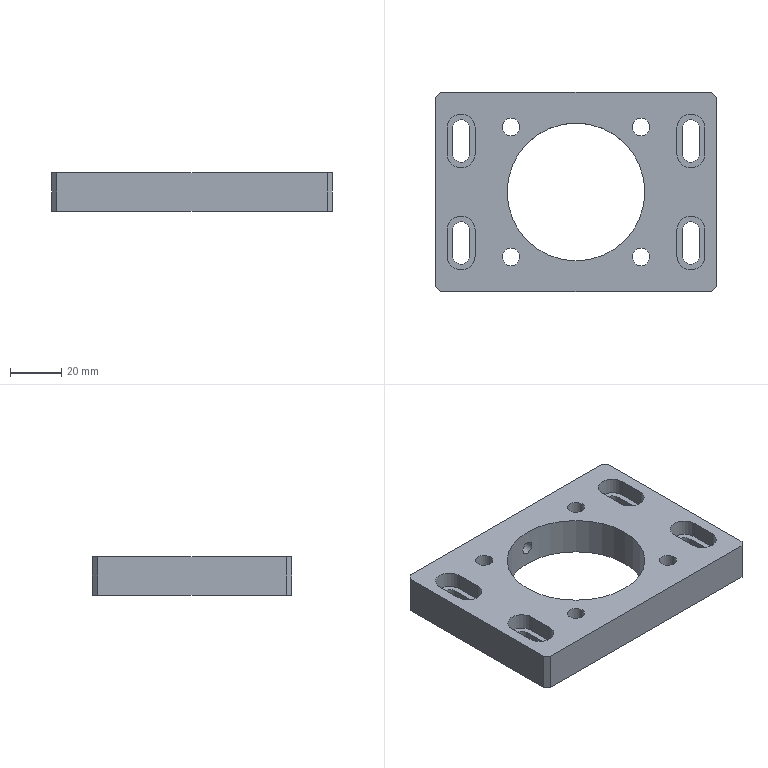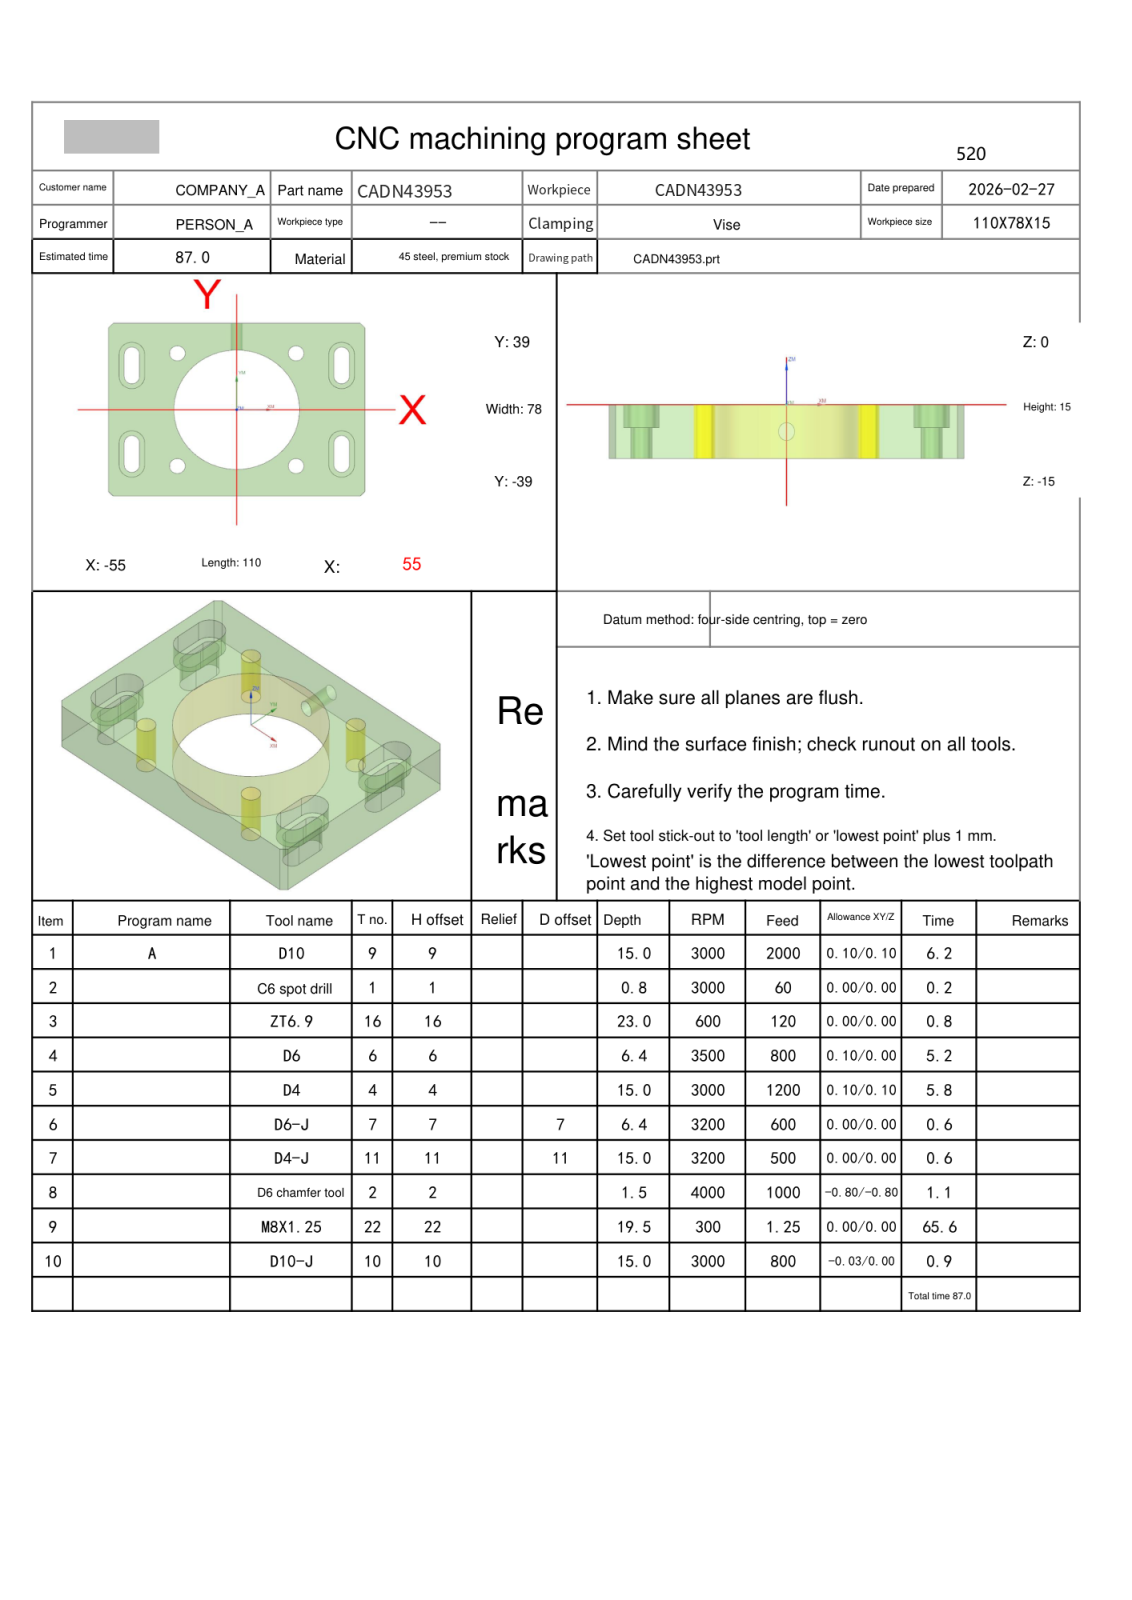NC program | NX | posted by the shop | part box 110 x 78 x 15 mm
Lines 1525 to 2257 of 4469:
N4 T06 M06
(D6  D=6. R=0. H=06 ce=0.10 di=0.00)
G00 G90 G54 X-47.4 Y-20. M03 S3500
G43 H06 Z50.
M08
Z.5
G01 Y-25. Z.465 F800.
G03 X-45. Y-27.4 Z.438 I2.4 J0.0
X-42.6 Y-25. Z.412 I0.0 J2.4
G01 Y-15. Z.342
G03 X-45. Y-12.6 Z.315 I-2.4 J0.0
X-47.4 Y-15. Z.289 I0.0 J-2.4
G01 Y-25. Z.218
G03 X-45. Y-27.4 Z.192 I2.4 J0.0
X-42.6 Y-25. Z.165 I0.0 J2.4
G01 Y-15. Z.095
G03 X-45. Y-12.6 Z.069 I-2.4 J0.0
X-47.4 Y-15. Z.042 I0.0 J-2.4
G01 Y-25. Z-.028
G03 X-45. Y-27.4 Z-.054 I2.4 J0.0
X-42.6 Y-25. Z-.081 I0.0 J2.4
G01 Y-15. Z-.151
G03 X-45. Y-12.6 Z-.178 I-2.4 J0.0
X-47.4 Y-15. Z-.204 I0.0 J-2.4
G01 Y-25. Z-.274
G03 X-45. Y-27.4 Z-.301 I2.4 J0.0
X-42.6 Y-25. Z-.327 I0.0 J2.4
G01 Y-15. Z-.398
G03 X-45. Y-12.6 Z-.424 I-2.4 J0.0
X-47.4 Y-15. Z-.451 I0.0 J-2.4
G01 Y-25. Z-.521
G03 X-45. Y-27.4 Z-.547 I2.4 J0.0
X-42.6 Y-25. Z-.574 I0.0 J2.4
G01 Y-15. Z-.644
G03 X-45. Y-12.6 Z-.671 I-2.4 J0.0
X-47.4 Y-15. Z-.697 I0.0 J-2.4
G01 Y-25. Z-.767
G03 X-45. Y-27.4 Z-.794 I2.4 J0.0
X-42.6 Y-25. Z-.82 I0.0 J2.4
G01 Y-15. Z-.89
G03 X-45. Y-12.6 Z-.917 I-2.4 J0.0
X-47.4 Y-15. Z-.943 I0.0 J-2.4
G01 Y-25. Z-1.014
G03 X-45. Y-27.4 Z-1.04 I2.4 J0.0
X-42.6 Y-25. Z-1.067 I0.0 J2.4
G01 Y-15. Z-1.137
G03 X-45. Y-12.6 Z-1.163 I-2.4 J0.0
X-47.4 Y-15. Z-1.19 I0.0 J-2.4
G01 Y-25. Z-1.26
G03 X-45. Y-27.4 Z-1.287 I2.4 J0.0
X-42.6 Y-25. Z-1.313 I0.0 J2.4
G01 Y-15. Z-1.383
G03 X-45. Y-12.6 Z-1.41 I-2.4 J0.0
X-47.4 Y-15. Z-1.436 I0.0 J-2.4
G01 Y-25. Z-1.507
G03 X-45. Y-27.4 Z-1.533 I2.4 J0.0
X-42.6 Y-25. Z-1.56 I0.0 J2.4
G01 Y-15. Z-1.63
G03 X-45. Y-12.6 Z-1.656 I-2.4 J0.0
X-47.4 Y-15. Z-1.683 I0.0 J-2.4
G01 Y-25. Z-1.753
G03 X-45. Y-27.4 Z-1.779 I2.4 J0.0
X-42.6 Y-25. Z-1.806 I0.0 J2.4
G01 Y-15. Z-1.876
G03 X-45. Y-12.6 Z-1.903 I-2.4 J0.0
X-47.4 Y-15. Z-1.929 I0.0 J-2.4
G01 Y-25. Z-1.999
G03 X-45. Y-27.4 Z-2.026 I2.4 J0.0
X-42.6 Y-25. Z-2.052 I0.0 J2.4
G01 Y-15. Z-2.123
G03 X-45. Y-12.6 Z-2.149 I-2.4 J0.0
X-47.4 Y-15. Z-2.176 I0.0 J-2.4
G01 Y-25. Z-2.246
G03 X-45. Y-27.4 Z-2.272 I2.4 J0.0
X-42.6 Y-25. Z-2.299 I0.0 J2.4
G01 Y-15. Z-2.369
G03 X-45. Y-12.6 Z-2.396 I-2.4 J0.0
X-47.4 Y-15. Z-2.422 I0.0 J-2.4
G01 Y-25. Z-2.492
G03 X-45. Y-27.4 Z-2.519 I2.4 J0.0
X-42.6 Y-25. Z-2.545 I0.0 J2.4
G01 Y-15. Z-2.615
G03 X-45. Y-12.6 Z-2.642 I-2.4 J0.0
X-47.4 Y-15. Z-2.668 I0.0 J-2.4
G01 Y-25. Z-2.739
G03 X-45. Y-27.4 Z-2.765 I2.4 J0.0
X-42.6 Y-25. Z-2.792 I0.0 J2.4
G01 Y-15. Z-2.862
G03 X-45. Y-12.6 Z-2.888 I-2.4 J0.0
X-47.4 Y-15. Z-2.915 I0.0 J-2.4
G01 Y-25. Z-2.985
G03 X-45. Y-27.4 Z-3.012 I2.4 J0.0
X-42.6 Y-25. Z-3.038 I0.0 J2.4
G01 Y-15. Z-3.108
G03 X-45. Y-12.6 Z-3.135 I-2.4 J0.0
X-47.4 Y-15. Z-3.161 I0.0 J-2.4
G01 Y-25. Z-3.232
G03 X-45. Y-27.4 Z-3.258 I2.4 J0.0
X-42.6 Y-25. Z-3.285 I0.0 J2.4
G01 Y-15. Z-3.355
G03 X-45. Y-12.6 Z-3.381 I-2.4 J0.0
X-47.4 Y-15. Z-3.408 I0.0 J-2.4
G01 Y-25. Z-3.478
G03 X-45. Y-27.4 Z-3.504 I2.4 J0.0
X-42.6 Y-25. Z-3.531 I0.0 J2.4
G01 Y-15. Z-3.601
G03 X-45. Y-12.6 Z-3.628 I-2.4 J0.0
X-47.4 Y-15. Z-3.654 I0.0 J-2.4
G01 Y-25. Z-3.724
G03 X-45. Y-27.4 Z-3.751 I2.4 J0.0
X-42.6 Y-25. Z-3.777 I0.0 J2.4
G01 Y-15. Z-3.848
G03 X-45. Y-12.6 Z-3.874 I-2.4 J0.0
X-47.4 Y-15. Z-3.901 I0.0 J-2.4
G01 Y-25. Z-3.971
G03 X-45. Y-27.4 Z-3.997 I2.4 J0.0
X-42.6 Y-25. Z-4.024 I0.0 J2.4
G01 Y-15. Z-4.094
G03 X-45. Y-12.6 Z-4.121 I-2.4 J0.0
X-47.4 Y-15. Z-4.147 I0.0 J-2.4
G01 Y-25. Z-4.217
G03 X-45. Y-27.4 Z-4.244 I2.4 J0.0
X-42.6 Y-25. Z-4.27 I0.0 J2.4
G01 Y-15. Z-4.34
G03 X-45. Y-12.6 Z-4.367 I-2.4 J0.0
X-47.4 Y-15. Z-4.393 I0.0 J-2.4
G01 Y-25. Z-4.464
G03 X-45. Y-27.4 Z-4.49 I2.4 J0.0
X-42.6 Y-25. Z-4.517 I0.0 J2.4
G01 Y-15. Z-4.587
G03 X-45. Y-12.6 Z-4.613 I-2.4 J0.0
X-47.4 Y-15. Z-4.64 I0.0 J-2.4
G01 Y-25. Z-4.71
G03 X-45. Y-27.4 Z-4.737 I2.4 J0.0
X-42.6 Y-25. Z-4.763 I0.0 J2.4
G01 Y-15. Z-4.833
G03 X-45. Y-12.6 Z-4.86 I-2.4 J0.0
X-47.4 Y-15. Z-4.886 I0.0 J-2.4
G01 Y-25. Z-4.957
G03 X-45. Y-27.4 Z-4.983 I2.4 J0.0
X-42.6 Y-25. Z-5.01 I0.0 J2.4
G01 Y-15. Z-5.08
G03 X-45. Y-12.6 Z-5.106 I-2.4 J0.0
X-47.4 Y-15. Z-5.133 I0.0 J-2.4
G01 Y-25. Z-5.203
G03 X-45. Y-27.4 Z-5.229 I2.4 J0.0
X-42.6 Y-25. Z-5.256 I0.0 J2.4
G01 Y-15. Z-5.326
G03 X-45. Y-12.6 Z-5.353 I-2.4 J0.0
X-47.4 Y-15. Z-5.379 I0.0 J-2.4
G01 Y-25. Z-5.449
G03 X-45. Y-27.4 Z-5.476 I2.4 J0.0
X-42.6 Y-25. Z-5.502 I0.0 J2.4
G01 Y-15. Z-5.573
G03 X-45. Y-12.6 Z-5.599 I-2.4 J0.0
X-47.4 Y-15. Z-5.626 I0.0 J-2.4
G01 Y-25. Z-5.696
G03 X-45. Y-27.4 Z-5.722 I2.4 J0.0
X-42.6 Y-25. Z-5.749 I0.0 J2.4
G01 Y-15. Z-5.819
G03 X-45. Y-12.6 Z-5.846 I-2.4 J0.0
X-47.4 Y-15. Z-5.872 I0.0 J-2.4
G01 Y-25. Z-5.942
G03 X-45. Y-27.4 Z-5.969 I2.4 J0.0
X-42.6 Y-25. Z-5.995 I0.0 J2.4
G01 Y-15. Z-6.065
G03 X-45. Y-12.6 Z-6.092 I-2.4 J0.0
X-47.4 Y-15. Z-6.118 I0.0 J-2.4
G01 Y-25. Z-6.189
G03 X-45. Y-27.4 Z-6.215 I2.4 J0.0
X-42.6 Y-25. Z-6.242 I0.0 J2.4
G01 Y-15. Z-6.312
G03 X-45. Y-12.6 Z-6.338 I-2.4 J0.0
X-47.4 Y-15. Z-6.365 I0.0 J-2.4
G01 Y-20. Z-6.4
Y-25.
G03 X-45. Y-27.4 I2.4 J0.0
X-42.6 Y-25. I0.0 J2.4
G01 Y-15.
G03 X-45. Y-12.6 I-2.4 J0.0
X-47.4 Y-15. I0.0 J-2.4
G01 Y-20.
Y-20.5
Z-5.4
G00 Z50.
Y20.
Z.5
G01 Y15. Z.465
G03 X-45. Y12.6 Z.438 I2.4 J0.0
X-42.6 Y15. Z.412 I0.0 J2.4
G01 Y25. Z.342
G03 X-45. Y27.4 Z.315 I-2.4 J0.0
X-47.4 Y25. Z.289 I0.0 J-2.4
G01 Y15. Z.218
G03 X-45. Y12.6 Z.192 I2.4 J0.0
X-42.6 Y15. Z.165 I0.0 J2.4
G01 Y25. Z.095
G03 X-45. Y27.4 Z.069 I-2.4 J0.0
X-47.4 Y25. Z.042 I0.0 J-2.4
G01 Y15. Z-.028
G03 X-45. Y12.6 Z-.054 I2.4 J0.0
X-42.6 Y15. Z-.081 I0.0 J2.4
G01 Y25. Z-.151
G03 X-45. Y27.4 Z-.178 I-2.4 J0.0
X-47.4 Y25. Z-.204 I0.0 J-2.4
G01 Y15. Z-.274
G03 X-45. Y12.6 Z-.301 I2.4 J0.0
X-42.6 Y15. Z-.327 I0.0 J2.4
G01 Y25. Z-.398
G03 X-45. Y27.4 Z-.424 I-2.4 J0.0
X-47.4 Y25. Z-.451 I0.0 J-2.4
G01 Y15. Z-.521
G03 X-45. Y12.6 Z-.547 I2.4 J0.0
X-42.6 Y15. Z-.574 I0.0 J2.4
G01 Y25. Z-.644
G03 X-45. Y27.4 Z-.671 I-2.4 J0.0
X-47.4 Y25. Z-.697 I0.0 J-2.4
G01 Y15. Z-.767
G03 X-45. Y12.6 Z-.794 I2.4 J0.0
X-42.6 Y15. Z-.82 I0.0 J2.4
G01 Y25. Z-.89
G03 X-45. Y27.4 Z-.917 I-2.4 J0.0
X-47.4 Y25. Z-.943 I0.0 J-2.4
G01 Y15. Z-1.014
G03 X-45. Y12.6 Z-1.04 I2.4 J0.0
X-42.6 Y15. Z-1.067 I0.0 J2.4
G01 Y25. Z-1.137
G03 X-45. Y27.4 Z-1.163 I-2.4 J0.0
X-47.4 Y25. Z-1.19 I0.0 J-2.4
G01 Y15. Z-1.26
G03 X-45. Y12.6 Z-1.287 I2.4 J0.0
X-42.6 Y15. Z-1.313 I0.0 J2.4
G01 Y25. Z-1.383
G03 X-45. Y27.4 Z-1.41 I-2.4 J0.0
X-47.4 Y25. Z-1.436 I0.0 J-2.4
G01 Y15. Z-1.507
G03 X-45. Y12.6 Z-1.533 I2.4 J0.0
X-42.6 Y15. Z-1.56 I0.0 J2.4
G01 Y25. Z-1.63
G03 X-45. Y27.4 Z-1.656 I-2.4 J0.0
X-47.4 Y25. Z-1.683 I0.0 J-2.4
G01 Y15. Z-1.753
G03 X-45. Y12.6 Z-1.779 I2.4 J0.0
X-42.6 Y15. Z-1.806 I0.0 J2.4
G01 Y25. Z-1.876
G03 X-45. Y27.4 Z-1.903 I-2.4 J0.0
X-47.4 Y25. Z-1.929 I0.0 J-2.4
G01 Y15. Z-1.999
G03 X-45. Y12.6 Z-2.026 I2.4 J0.0
X-42.6 Y15. Z-2.052 I0.0 J2.4
G01 Y25. Z-2.123
G03 X-45. Y27.4 Z-2.149 I-2.4 J0.0
X-47.4 Y25. Z-2.176 I0.0 J-2.4
G01 Y15. Z-2.246
G03 X-45. Y12.6 Z-2.272 I2.4 J0.0
X-42.6 Y15. Z-2.299 I0.0 J2.4
G01 Y25. Z-2.369
G03 X-45. Y27.4 Z-2.396 I-2.4 J0.0
X-47.4 Y25. Z-2.422 I0.0 J-2.4
G01 Y15. Z-2.492
G03 X-45. Y12.6 Z-2.519 I2.4 J0.0
X-42.6 Y15. Z-2.545 I0.0 J2.4
G01 Y25. Z-2.615
G03 X-45. Y27.4 Z-2.642 I-2.4 J0.0
X-47.4 Y25. Z-2.668 I0.0 J-2.4
G01 Y15. Z-2.739
G03 X-45. Y12.6 Z-2.765 I2.4 J0.0
X-42.6 Y15. Z-2.792 I0.0 J2.4
G01 Y25. Z-2.862
G03 X-45. Y27.4 Z-2.888 I-2.4 J0.0
X-47.4 Y25. Z-2.915 I0.0 J-2.4
G01 Y15. Z-2.985
G03 X-45. Y12.6 Z-3.012 I2.4 J0.0
X-42.6 Y15. Z-3.038 I0.0 J2.4
G01 Y25. Z-3.108
G03 X-45. Y27.4 Z-3.135 I-2.4 J0.0
X-47.4 Y25. Z-3.161 I0.0 J-2.4
G01 Y15. Z-3.232
G03 X-45. Y12.6 Z-3.258 I2.4 J0.0
X-42.6 Y15. Z-3.285 I0.0 J2.4
G01 Y25. Z-3.355
G03 X-45. Y27.4 Z-3.381 I-2.4 J0.0
X-47.4 Y25. Z-3.408 I0.0 J-2.4
G01 Y15. Z-3.478
G03 X-45. Y12.6 Z-3.504 I2.4 J0.0
X-42.6 Y15. Z-3.531 I0.0 J2.4
G01 Y25. Z-3.601
G03 X-45. Y27.4 Z-3.628 I-2.4 J0.0
X-47.4 Y25. Z-3.654 I0.0 J-2.4
G01 Y15. Z-3.724
G03 X-45. Y12.6 Z-3.751 I2.4 J0.0
X-42.6 Y15. Z-3.777 I0.0 J2.4
G01 Y25. Z-3.848
G03 X-45. Y27.4 Z-3.874 I-2.4 J0.0
X-47.4 Y25. Z-3.901 I0.0 J-2.4
G01 Y15. Z-3.971
G03 X-45. Y12.6 Z-3.997 I2.4 J0.0
X-42.6 Y15. Z-4.024 I0.0 J2.4
G01 Y25. Z-4.094
G03 X-45. Y27.4 Z-4.121 I-2.4 J0.0
X-47.4 Y25. Z-4.147 I0.0 J-2.4
G01 Y15. Z-4.217
G03 X-45. Y12.6 Z-4.244 I2.4 J0.0
X-42.6 Y15. Z-4.27 I0.0 J2.4
G01 Y25. Z-4.34
G03 X-45. Y27.4 Z-4.367 I-2.4 J0.0
X-47.4 Y25. Z-4.393 I0.0 J-2.4
G01 Y15. Z-4.464
G03 X-45. Y12.6 Z-4.49 I2.4 J0.0
X-42.6 Y15. Z-4.517 I0.0 J2.4
G01 Y25. Z-4.587
G03 X-45. Y27.4 Z-4.613 I-2.4 J0.0
X-47.4 Y25. Z-4.64 I0.0 J-2.4
G01 Y15. Z-4.71
G03 X-45. Y12.6 Z-4.737 I2.4 J0.0
X-42.6 Y15. Z-4.763 I0.0 J2.4
G01 Y25. Z-4.833
G03 X-45. Y27.4 Z-4.86 I-2.4 J0.0
X-47.4 Y25. Z-4.886 I0.0 J-2.4
G01 Y15. Z-4.957
G03 X-45. Y12.6 Z-4.983 I2.4 J0.0
X-42.6 Y15. Z-5.01 I0.0 J2.4
G01 Y25. Z-5.08
G03 X-45. Y27.4 Z-5.106 I-2.4 J0.0
X-47.4 Y25. Z-5.133 I0.0 J-2.4
G01 Y15. Z-5.203
G03 X-45. Y12.6 Z-5.229 I2.4 J0.0
X-42.6 Y15. Z-5.256 I0.0 J2.4
G01 Y25. Z-5.326
G03 X-45. Y27.4 Z-5.353 I-2.4 J0.0
X-47.4 Y25. Z-5.379 I0.0 J-2.4
G01 Y15. Z-5.449
G03 X-45. Y12.6 Z-5.476 I2.4 J0.0
X-42.6 Y15. Z-5.502 I0.0 J2.4
G01 Y25. Z-5.573
G03 X-45. Y27.4 Z-5.599 I-2.4 J0.0
X-47.4 Y25. Z-5.626 I0.0 J-2.4
G01 Y15. Z-5.696
G03 X-45. Y12.6 Z-5.722 I2.4 J0.0
X-42.6 Y15. Z-5.749 I0.0 J2.4
G01 Y25. Z-5.819
G03 X-45. Y27.4 Z-5.846 I-2.4 J0.0
X-47.4 Y25. Z-5.872 I0.0 J-2.4
G01 Y15. Z-5.942
G03 X-45. Y12.6 Z-5.969 I2.4 J0.0
X-42.6 Y15. Z-5.995 I0.0 J2.4
G01 Y25. Z-6.065
G03 X-45. Y27.4 Z-6.092 I-2.4 J0.0
X-47.4 Y25. Z-6.118 I0.0 J-2.4
G01 Y15. Z-6.189
G03 X-45. Y12.6 Z-6.215 I2.4 J0.0
X-42.6 Y15. Z-6.242 I0.0 J2.4
G01 Y25. Z-6.312
G03 X-45. Y27.4 Z-6.338 I-2.4 J0.0
X-47.4 Y25. Z-6.365 I0.0 J-2.4
G01 Y20. Z-6.4
Y15.
G03 X-45. Y12.6 I2.4 J0.0
X-42.6 Y15. I0.0 J2.4
G01 Y25.
G03 X-45. Y27.4 I-2.4 J0.0
X-47.4 Y25. I0.0 J-2.4
G01 Y20.
Y19.5
Z-5.4
G00 Z50.
X47.4 Y20.
Z.5
G01 Y25. Z.465
G03 X45. Y27.4 Z.438 I-2.4 J0.0
X42.6 Y25. Z.412 I0.0 J-2.4
G01 Y15. Z.342
G03 X45. Y12.6 Z.315 I2.4 J0.0
X47.4 Y15. Z.289 I0.0 J2.4
G01 Y25. Z.218
G03 X45. Y27.4 Z.192 I-2.4 J0.0
X42.6 Y25. Z.165 I0.0 J-2.4
G01 Y15. Z.095
G03 X45. Y12.6 Z.069 I2.4 J0.0
X47.4 Y15. Z.042 I0.0 J2.4
G01 Y25. Z-.028
G03 X45. Y27.4 Z-.054 I-2.4 J0.0
X42.6 Y25. Z-.081 I0.0 J-2.4
G01 Y15. Z-.151
G03 X45. Y12.6 Z-.178 I2.4 J0.0
X47.4 Y15. Z-.204 I0.0 J2.4
G01 Y25. Z-.274
G03 X45. Y27.4 Z-.301 I-2.4 J0.0
X42.6 Y25. Z-.327 I0.0 J-2.4
G01 Y15. Z-.398
G03 X45. Y12.6 Z-.424 I2.4 J0.0
X47.4 Y15. Z-.451 I0.0 J2.4
G01 Y25. Z-.521
G03 X45. Y27.4 Z-.547 I-2.4 J0.0
X42.6 Y25. Z-.574 I0.0 J-2.4
G01 Y15. Z-.644
G03 X45. Y12.6 Z-.671 I2.4 J0.0
X47.4 Y15. Z-.697 I0.0 J2.4
G01 Y25. Z-.767
G03 X45. Y27.4 Z-.794 I-2.4 J0.0
X42.6 Y25. Z-.82 I0.0 J-2.4
G01 Y15. Z-.89
G03 X45. Y12.6 Z-.917 I2.4 J0.0
X47.4 Y15. Z-.943 I0.0 J2.4
G01 Y25. Z-1.014
G03 X45. Y27.4 Z-1.04 I-2.4 J0.0
X42.6 Y25. Z-1.067 I0.0 J-2.4
G01 Y15. Z-1.137
G03 X45. Y12.6 Z-1.163 I2.4 J0.0
X47.4 Y15. Z-1.19 I0.0 J2.4
G01 Y25. Z-1.26
G03 X45. Y27.4 Z-1.287 I-2.4 J0.0
X42.6 Y25. Z-1.313 I0.0 J-2.4
G01 Y15. Z-1.383
G03 X45. Y12.6 Z-1.41 I2.4 J0.0
X47.4 Y15. Z-1.436 I0.0 J2.4
G01 Y25. Z-1.507
G03 X45. Y27.4 Z-1.533 I-2.4 J0.0
X42.6 Y25. Z-1.56 I0.0 J-2.4
G01 Y15. Z-1.63
G03 X45. Y12.6 Z-1.656 I2.4 J0.0
X47.4 Y15. Z-1.683 I0.0 J2.4
G01 Y25. Z-1.753
G03 X45. Y27.4 Z-1.779 I-2.4 J0.0
X42.6 Y25. Z-1.806 I0.0 J-2.4
G01 Y15. Z-1.876
G03 X45. Y12.6 Z-1.903 I2.4 J0.0
X47.4 Y15. Z-1.929 I0.0 J2.4
G01 Y25. Z-1.999
G03 X45. Y27.4 Z-2.026 I-2.4 J0.0
X42.6 Y25. Z-2.052 I0.0 J-2.4
G01 Y15. Z-2.123
G03 X45. Y12.6 Z-2.149 I2.4 J0.0
X47.4 Y15. Z-2.176 I0.0 J2.4
G01 Y25. Z-2.246
G03 X45. Y27.4 Z-2.272 I-2.4 J0.0
X42.6 Y25. Z-2.299 I0.0 J-2.4
G01 Y15. Z-2.369
G03 X45. Y12.6 Z-2.396 I2.4 J0.0
X47.4 Y15. Z-2.422 I0.0 J2.4
G01 Y25. Z-2.492
G03 X45. Y27.4 Z-2.519 I-2.4 J0.0
X42.6 Y25. Z-2.545 I0.0 J-2.4
G01 Y15. Z-2.615
G03 X45. Y12.6 Z-2.642 I2.4 J0.0
X47.4 Y15. Z-2.668 I0.0 J2.4
G01 Y25. Z-2.739
G03 X45. Y27.4 Z-2.765 I-2.4 J0.0
X42.6 Y25. Z-2.792 I0.0 J-2.4
G01 Y15. Z-2.862
G03 X45. Y12.6 Z-2.888 I2.4 J0.0
X47.4 Y15. Z-2.915 I0.0 J2.4
G01 Y25. Z-2.985
G03 X45. Y27.4 Z-3.012 I-2.4 J0.0
X42.6 Y25. Z-3.038 I0.0 J-2.4
G01 Y15. Z-3.108
G03 X45. Y12.6 Z-3.135 I2.4 J0.0
X47.4 Y15. Z-3.161 I0.0 J2.4
G01 Y25. Z-3.232
G03 X45. Y27.4 Z-3.258 I-2.4 J0.0
X42.6 Y25. Z-3.285 I0.0 J-2.4
G01 Y15. Z-3.355
G03 X45. Y12.6 Z-3.381 I2.4 J0.0
X47.4 Y15. Z-3.408 I0.0 J2.4
G01 Y25. Z-3.478
G03 X45. Y27.4 Z-3.504 I-2.4 J0.0
X42.6 Y25. Z-3.531 I0.0 J-2.4
G01 Y15. Z-3.601
G03 X45. Y12.6 Z-3.628 I2.4 J0.0
X47.4 Y15. Z-3.654 I0.0 J2.4
G01 Y25. Z-3.724
G03 X45. Y27.4 Z-3.751 I-2.4 J0.0
X42.6 Y25. Z-3.777 I0.0 J-2.4
G01 Y15. Z-3.848
G03 X45. Y12.6 Z-3.874 I2.4 J0.0
X47.4 Y15. Z-3.901 I0.0 J2.4
G01 Y25. Z-3.971
G03 X45. Y27.4 Z-3.997 I-2.4 J0.0
X42.6 Y25. Z-4.024 I0.0 J-2.4
G01 Y15. Z-4.094
G03 X45. Y12.6 Z-4.121 I2.4 J0.0
X47.4 Y15. Z-4.147 I0.0 J2.4
G01 Y25. Z-4.217
G03 X45. Y27.4 Z-4.244 I-2.4 J0.0
X42.6 Y25. Z-4.27 I0.0 J-2.4
G01 Y15. Z-4.34
G03 X45. Y12.6 Z-4.367 I2.4 J0.0
X47.4 Y15. Z-4.393 I0.0 J2.4
G01 Y25. Z-4.464
G03 X45. Y27.4 Z-4.49 I-2.4 J0.0
X42.6 Y25. Z-4.517 I0.0 J-2.4
G01 Y15. Z-4.587
G03 X45. Y12.6 Z-4.613 I2.4 J0.0
X47.4 Y15. Z-4.64 I0.0 J2.4
G01 Y25. Z-4.71
G03 X45. Y27.4 Z-4.737 I-2.4 J0.0
X42.6 Y25. Z-4.763 I0.0 J-2.4
G01 Y15. Z-4.833
G03 X45. Y12.6 Z-4.86 I2.4 J0.0
X47.4 Y15. Z-4.886 I0.0 J2.4
G01 Y25. Z-4.957
G03 X45. Y27.4 Z-4.983 I-2.4 J0.0
X42.6 Y25. Z-5.01 I0.0 J-2.4
G01 Y15. Z-5.08
G03 X45. Y12.6 Z-5.106 I2.4 J0.0
X47.4 Y15. Z-5.133 I0.0 J2.4
G01 Y25. Z-5.203
G03 X45. Y27.4 Z-5.229 I-2.4 J0.0
X42.6 Y25. Z-5.256 I0.0 J-2.4
G01 Y15. Z-5.326
G03 X45. Y12.6 Z-5.353 I2.4 J0.0
X47.4 Y15. Z-5.379 I0.0 J2.4
G01 Y25. Z-5.449
G03 X45. Y27.4 Z-5.476 I-2.4 J0.0
X42.6 Y25. Z-5.502 I0.0 J-2.4
G01 Y15. Z-5.573
G03 X45. Y12.6 Z-5.599 I2.4 J0.0
X47.4 Y15. Z-5.626 I0.0 J2.4
G01 Y25. Z-5.696
G03 X45. Y27.4 Z-5.722 I-2.4 J0.0
X42.6 Y25. Z-5.749 I0.0 J-2.4
G01 Y15. Z-5.819
G03 X45. Y12.6 Z-5.846 I2.4 J0.0
X47.4 Y15. Z-5.872 I0.0 J2.4
G01 Y25. Z-5.942
G03 X45. Y27.4 Z-5.969 I-2.4 J0.0
X42.6 Y25. Z-5.995 I0.0 J-2.4
G01 Y15. Z-6.065
G03 X45. Y12.6 Z-6.092 I2.4 J0.0
X47.4 Y15. Z-6.118 I0.0 J2.4
G01 Y25. Z-6.189
G03 X45. Y27.4 Z-6.215 I-2.4 J0.0
X42.6 Y25. Z-6.242 I0.0 J-2.4
G01 Y15. Z-6.312
G03 X45. Y12.6 Z-6.338 I2.4 J0.0
X47.4 Y15. Z-6.365 I0.0 J2.4
G01 Y20. Z-6.4
Y25.
G03 X45. Y27.4 I-2.4 J0.0
X42.6 Y25. I0.0 J-2.4
G01 Y15.
G03 X45. Y12.6 I2.4 J0.0
X47.4 Y15. I0.0 J2.4
G01 Y20.
Y20.5
Z-5.4
G00 Z50.
Y-20.
Z.5
G01 Y-15. Z.465
G03 X45. Y-12.6 Z.438 I-2.4 J0.0
X42.6 Y-15. Z.412 I0.0 J-2.4
G01 Y-25. Z.342
G03 X45. Y-27.4 Z.315 I2.4 J0.0
X47.4 Y-25. Z.289 I0.0 J2.4
G01 Y-15. Z.218
G03 X45. Y-12.6 Z.192 I-2.4 J0.0
X42.6 Y-15. Z.165 I0.0 J-2.4
G01 Y-25. Z.095
G03 X45. Y-27.4 Z.069 I2.4 J0.0
X47.4 Y-25. Z.042 I0.0 J2.4
G01 Y-15. Z-.028
G03 X45. Y-12.6 Z-.054 I-2.4 J0.0
X42.6 Y-15. Z-.081 I0.0 J-2.4
G01 Y-25. Z-.151
G03 X45. Y-27.4 Z-.178 I2.4 J0.0
X47.4 Y-25. Z-.204 I0.0 J2.4
G01 Y-15. Z-.274
G03 X45. Y-12.6 Z-.301 I-2.4 J0.0
X42.6 Y-15. Z-.327 I0.0 J-2.4
G01 Y-25. Z-.398
G03 X45. Y-27.4 Z-.424 I2.4 J0.0
X47.4 Y-25. Z-.451 I0.0 J2.4
G01 Y-15. Z-.521
G03 X45. Y-12.6 Z-.547 I-2.4 J0.0
X42.6 Y-15. Z-.574 I0.0 J-2.4
G01 Y-25. Z-.644
G03 X45. Y-27.4 Z-.671 I2.4 J0.0
X47.4 Y-25. Z-.697 I0.0 J2.4
G01 Y-15. Z-.767
G03 X45. Y-12.6 Z-.794 I-2.4 J0.0
X42.6 Y-15. Z-.82 I0.0 J-2.4
G01 Y-25. Z-.89
G03 X45. Y-27.4 Z-.917 I2.4 J0.0
X47.4 Y-25. Z-.943 I0.0 J2.4
G01 Y-15. Z-1.014
G03 X45. Y-12.6 Z-1.04 I-2.4 J0.0
X42.6 Y-15. Z-1.067 I0.0 J-2.4
G01 Y-25. Z-1.137
G03 X45. Y-27.4 Z-1.163 I2.4 J0.0
X47.4 Y-25. Z-1.19 I0.0 J2.4
G01 Y-15. Z-1.26
G03 X45. Y-12.6 Z-1.287 I-2.4 J0.0
X42.6 Y-15. Z-1.313 I0.0 J-2.4
G01 Y-25. Z-1.383
G03 X45. Y-27.4 Z-1.41 I2.4 J0.0
X47.4 Y-25. Z-1.436 I0.0 J2.4
G01 Y-15. Z-1.507
G03 X45. Y-12.6 Z-1.533 I-2.4 J0.0
X42.6 Y-15. Z-1.56 I0.0 J-2.4
G01 Y-25. Z-1.63
G03 X45. Y-27.4 Z-1.656 I2.4 J0.0
X47.4 Y-25. Z-1.683 I0.0 J2.4
G01 Y-15. Z-1.753
G03 X45. Y-12.6 Z-1.779 I-2.4 J0.0
X42.6 Y-15. Z-1.806 I0.0 J-2.4
G01 Y-25. Z-1.876
G03 X45. Y-27.4 Z-1.903 I2.4 J0.0
X47.4 Y-25. Z-1.929 I0.0 J2.4
G01 Y-15. Z-1.999
G03 X45. Y-12.6 Z-2.026 I-2.4 J0.0
X42.6 Y-15. Z-2.052 I0.0 J-2.4
G01 Y-25. Z-2.123
G03 X45. Y-27.4 Z-2.149 I2.4 J0.0
X47.4 Y-25. Z-2.176 I0.0 J2.4
G01 Y-15. Z-2.246
G03 X45. Y-12.6 Z-2.272 I-2.4 J0.0
X42.6 Y-15. Z-2.299 I0.0 J-2.4
G01 Y-25. Z-2.369
G03 X45. Y-27.4 Z-2.396 I2.4 J0.0
X47.4 Y-25. Z-2.422 I0.0 J2.4
G01 Y-15. Z-2.492
G03 X45. Y-12.6 Z-2.519 I-2.4 J0.0
X42.6 Y-15. Z-2.545 I0.0 J-2.4
G01 Y-25. Z-2.615
G03 X45. Y-27.4 Z-2.642 I2.4 J0.0
X47.4 Y-25. Z-2.668 I0.0 J2.4
G01 Y-15. Z-2.739
G03 X45. Y-12.6 Z-2.765 I-2.4 J0.0
X42.6 Y-15. Z-2.792 I0.0 J-2.4
G01 Y-25. Z-2.862
G03 X45. Y-27.4 Z-2.888 I2.4 J0.0
X47.4 Y-25. Z-2.915 I0.0 J2.4
G01 Y-15. Z-2.985
G03 X45. Y-12.6 Z-3.012 I-2.4 J0.0
X42.6 Y-15. Z-3.038 I0.0 J-2.4
G01 Y-25. Z-3.108
G03 X45. Y-27.4 Z-3.135 I2.4 J0.0
X47.4 Y-25. Z-3.161 I0.0 J2.4
G01 Y-15. Z-3.232
G03 X45. Y-12.6 Z-3.258 I-2.4 J0.0
X42.6 Y-15. Z-3.285 I0.0 J-2.4
G01 Y-25. Z-3.355
G03 X45. Y-27.4 Z-3.381 I2.4 J0.0
X47.4 Y-25. Z-3.408 I0.0 J2.4
G01 Y-15. Z-3.478
G03 X45. Y-12.6 Z-3.504 I-2.4 J0.0
X42.6 Y-15. Z-3.531 I0.0 J-2.4
G01 Y-25. Z-3.601
G03 X45. Y-27.4 Z-3.628 I2.4 J0.0
X47.4 Y-25. Z-3.654 I0.0 J2.4
G01 Y-15. Z-3.724
G03 X45. Y-12.6 Z-3.751 I-2.4 J0.0
X42.6 Y-15. Z-3.777 I0.0 J-2.4
G01 Y-25. Z-3.848
G03 X45. Y-27.4 Z-3.874 I2.4 J0.0
X47.4 Y-25. Z-3.901 I0.0 J2.4
G01 Y-15. Z-3.971
G03 X45. Y-12.6 Z-3.997 I-2.4 J0.0
X42.6 Y-15. Z-4.024 I0.0 J-2.4
G01 Y-25. Z-4.094
G03 X45. Y-27.4 Z-4.121 I2.4 J0.0
X47.4 Y-25. Z-4.147 I0.0 J2.4
G01 Y-15. Z-4.217
G03 X45. Y-12.6 Z-4.244 I-2.4 J0.0
X42.6 Y-15. Z-4.27 I0.0 J-2.4
G01 Y-25. Z-4.34
G03 X45. Y-27.4 Z-4.367 I2.4 J0.0
X47.4 Y-25. Z-4.393 I0.0 J2.4
G01 Y-15. Z-4.464
G03 X45. Y-12.6 Z-4.49 I-2.4 J0.0
X42.6 Y-15. Z-4.517 I0.0 J-2.4
G01 Y-25. Z-4.587
G03 X45. Y-27.4 Z-4.613 I2.4 J0.0
X47.4 Y-25. Z-4.64 I0.0 J2.4
G01 Y-15. Z-4.71
G03 X45. Y-12.6 Z-4.737 I-2.4 J0.0
X42.6 Y-15. Z-4.763 I0.0 J-2.4
G01 Y-25. Z-4.833
G03 X45. Y-27.4 Z-4.86 I2.4 J0.0
X47.4 Y-25. Z-4.886 I0.0 J2.4
G01 Y-15. Z-4.957
G03 X45. Y-12.6 Z-4.983 I-2.4 J0.0
X42.6 Y-15. Z-5.01 I0.0 J-2.4
G01 Y-25. Z-5.08
G03 X45. Y-27.4 Z-5.106 I2.4 J0.0
X47.4 Y-25. Z-5.133 I0.0 J2.4
G01 Y-15. Z-5.203
G03 X45. Y-12.6 Z-5.229 I-2.4 J0.0
X42.6 Y-15. Z-5.256 I0.0 J-2.4
G01 Y-25. Z-5.326
G03 X45. Y-27.4 Z-5.353 I2.4 J0.0
X47.4 Y-25. Z-5.379 I0.0 J2.4
G01 Y-15. Z-5.449
G03 X45. Y-12.6 Z-5.476 I-2.4 J0.0
X42.6 Y-15. Z-5.502 I0.0 J-2.4
G01 Y-25. Z-5.573
G03 X45. Y-27.4 Z-5.599 I2.4 J0.0
X47.4 Y-25. Z-5.626 I0.0 J2.4
G01 Y-15. Z-5.696
G03 X45. Y-12.6 Z-5.722 I-2.4 J0.0
X42.6 Y-15. Z-5.749 I0.0 J-2.4
G01 Y-25. Z-5.819
G03 X45. Y-27.4 Z-5.846 I2.4 J0.0
X47.4 Y-25. Z-5.872 I0.0 J2.4
G01 Y-15. Z-5.942
G03 X45. Y-12.6 Z-5.969 I-2.4 J0.0
X42.6 Y-15. Z-5.995 I0.0 J-2.4
G01 Y-25. Z-6.065
G03 X45. Y-27.4 Z-6.092 I2.4 J0.0
X47.4 Y-25. Z-6.118 I0.0 J2.4
G01 Y-15. Z-6.189
G03 X45. Y-12.6 Z-6.215 I-2.4 J0.0
X42.6 Y-15. Z-6.242 I0.0 J-2.4
G01 Y-25. Z-6.312
G03 X45. Y-27.4 Z-6.338 I2.4 J0.0
X47.4 Y-25. Z-6.365 I0.0 J2.4
G01 Y-20. Z-6.4
Y-15.
G03 X45. Y-12.6 I-2.4 J0.0
X42.6 Y-15. I0.0 J-2.4
G01 Y-25.
G03 X45. Y-27.4 I2.4 J0.0
X47.4 Y-25. I0.0 J2.4
G01 Y-20.
Y-19.5
Z-5.4
G00 Z50.
G91 G28 Z0.0
M05
M09
G91 G28 Z0.0
M01